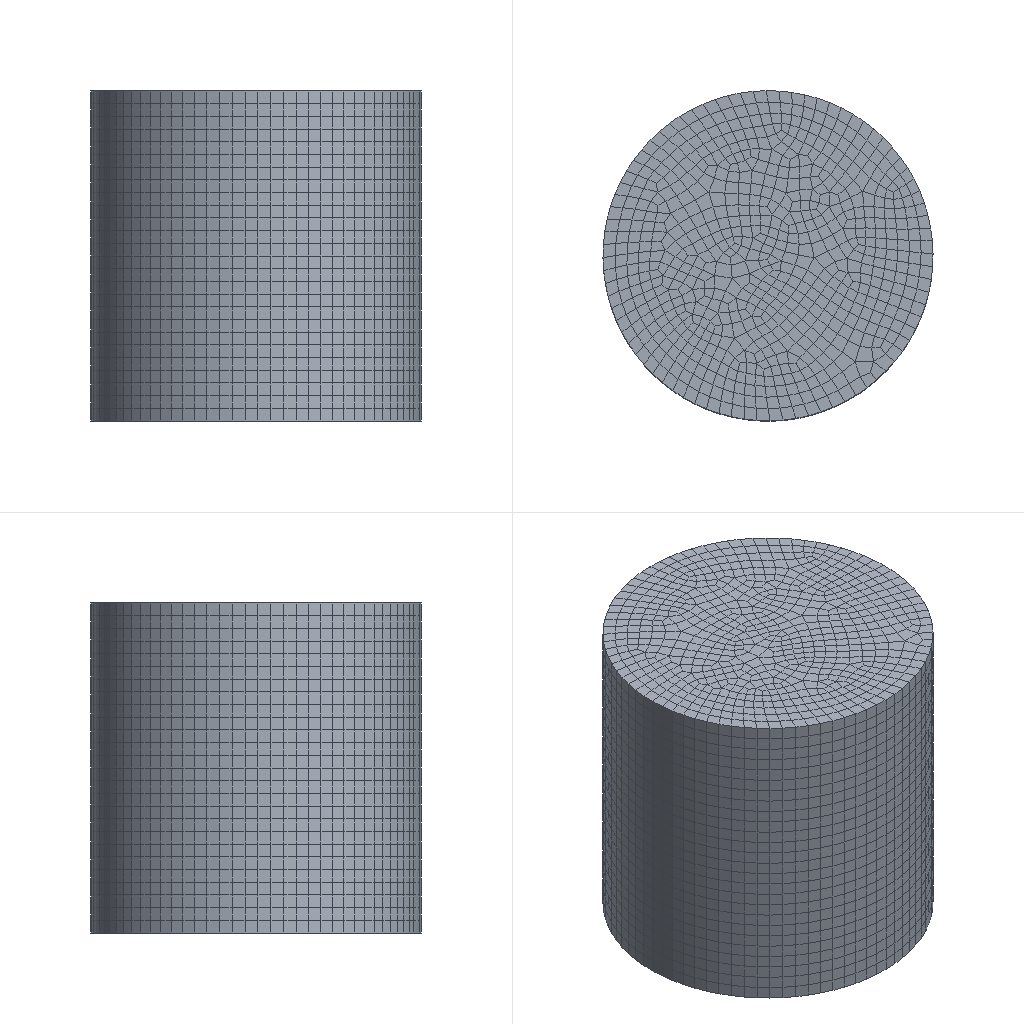Simulation study | abaqus
Set-up summary:
category,name,step,type,value,unit,region
solver,abaqus
solver,version,,,Abaqus/Standard 2020
units,not stated in the deck,,not stated
analysis,deck,,static,static
load_step,Step-1,Step-1,static
load_step,requested,,,1
mesh,nodes,,,20804
mesh,elements,,,18954
element_type,C3D8R,,solid,18252
element_type,COH3D8,,cohesive,702
load,load commands in deck,,count,1
bc,support commands in deck,,count,12
material,COH,,in results
material,MATERIAL-1,,in results
check,setup vs results,,match,"per instance, exact: element labels, types and connectivity; labels of the nodes the elements use; coordinates of those nodes at SINGLE_PRECISION in 1 of 1 instance(s)"
Abaqus input file, long lists of numbers shortened:
*Heading
** Job name: Job-1 Model name: Model-1
** Generated by: Abaqus/CAE 2020
*Preprint, echo=NO, model=NO, history=NO, contact=NO
**
** PARTS
**
*Part, name=Part-1
*Node
      1,   19.206,  -16.005,          25.
      2,   19.206,  -16.005,          50.
** (20802 more lines like these left out)
*Element, type=C3D8R
   1,  1575,  4160,  4244,  1574, 20062, 20063, 20064, 20065
   2,  4161,  1577,  1578,  4162, 20066, 20067, 20068, 20069
** (18250 more lines like these left out)
*Element, type=COH3D8
18253,    10,   335,   251,    11, 20065, 20064, 20063, 20062
18254,   253,    14,    13,   252, 20069, 20068, 20067, 20066
** (700 more lines like these left out)
*Nset, nset=Set-1, generate
     1,  20804,      1
*Elset, elset=Set-1, generate
     1,  18252,      1
*Elset, elset=CohesiveSeam-1-Elements, generate
 18253,  18954,      1
*Nset, nset=CohesiveSeam-1-TopNodes, generate
 20062,  20804,      1
*Nset, nset=CohesiveSeam-1-BottomNodes
   1,   4,   5,   6,   7,   8,   9,  10,  11,  12,  13,  14,  15,  16,  17,  18
  19,  20,  21,  22,  23,  24,  25,  26,  27,  28,  29,  30,  31,  32,  33,  34
** (45 more lines like these left out)
*Elset, elset=__PickedSurf8_S1, internal, generate
 18253,  18954,      1
*Surface, type=ELEMENT, name=_PickedSurf8, internal
__PickedSurf8_S1, S1
*Elset, elset=_CohesiveSeam-1-TopSurf_S2, internal, generate
 18253,  18954,      1
*Surface, type=ELEMENT, name=CohesiveSeam-1-TopSurf
_CohesiveSeam-1-TopSurf_S2, S2
*Elset, elset=_CohesiveSeam-1-BottomSurf_S1, internal, generate
 18253,  18954,      1
*Surface, type=ELEMENT, name=CohesiveSeam-1-BottomSurf
_CohesiveSeam-1-BottomSurf_S1, S1
** Section: Section-1
*Solid Section, elset=Set-1, material=Material-1
,
** Section: coh
*Cohesive Section, elset=CohesiveSeam-1-Elements, controls=EC-1, material=coh, response=TRACTION SEPARATION
,
*End Part
**
**
** ASSEMBLY
**
*Assembly, name=Assembly
**
*Instance, name=Part-1-1, part=Part-1
*End Instance
**
*Node
      1,           0., 1.53080845e-15,           0.
*Nset, nset=Set-1, instance=Part-1-1
    1,    3,    4,    5,    6,    7,    8,    9,   10,   11,   12,   13,   14,   15,   16,   17
   18,   19,   20,   21,   22,   23,   24,   25,   26,   27,   28,   29,   30,   31,   32,   33
** (68 more lines like these left out)
*Elset, elset=Set-1, instance=Part-1-1
  9127,  9128,  9129,  9130,  9131,  9132,  9133,  9134,  9136,  9137,  9138,  9140,  9141,  9143,  9144,  9145
  9147,  9148,  9150,  9151,  9152,  9153,  9154,  9155,  9156,  9159,  9160,  9162,  9163,  9164,  9166,  9167
** (63 more lines like these left out)
*Nset, nset=Set-2, instance=Part-1-1
     2,    83,    84,    85,    86,    87,    88,    89,    90,    91,    92,    93,    94,    95,    96,    97
    98,    99,   100,   101,   102,   103,   104,   105,   106,   107,   108,   109,   110,   111,   112,   113
** (68 more lines like these left out)
*Elset, elset=Set-2, instance=Part-1-1
    1,    2,    3,    4,    5,    6,    7,    8,   10,   11,   12,   14,   15,   17,   18,   19
   21,   22,   24,   25,   26,   27,   28,   29,   30,   33,   34,   36,   37,   38,   40,   41
** (63 more lines like these left out)
*Nset, nset=Set-3, instance=Part-1-1
    3,  162,  163,  164,  165,  166,  167,  168,  169,  170,  171,  172,  173,  174,  175,  176
  177,  178,  179,  180,  181,  182,  183,  184,  185,  186,  187,  188,  189,  190,  191,  192
** (45 more lines like these left out)
*Elset, elset=Set-3, instance=Part-1-1, generate
 17551,  18252,      1
*Nset, nset=Set-5
 1,
*Nset, nset=Set-6, instance=Part-1-1, generate
     1,  20804,      1
*Nset, nset=Set-6
 1,
*Elset, elset=Set-6, instance=Part-1-1, generate
     1,  18954,      1
*Nset, nset=m_Set-4
 1,
*Elset, elset=_s_Surf-1_S2, internal, instance=Part-1-1, generate
 17551,  18252,      1
*Surface, type=ELEMENT, name=s_Surf-1
_s_Surf-1_S2, S2
** Constraint: Constraint-1
*Coupling, constraint name=Constraint-1, ref node=m_Set-4, surface=s_Surf-1
*Kinematic
*Elset, elset=__Int-2_gcs0_2_S6, internal, instance=Part-1-1
    1,    4,   10,   11,   14,   18,   19,   22,   26,   33,   34,   40,   41,   44,   47,   48
   50,   51,   56,   57,   61,   63,   65,   83,  168,  703,  706,  712,  713,  716,  720,  721
** (19 more lines like these left out)
*Elset, elset=__Int-2_gcs0_2_S4, internal, instance=Part-1-1
    2,    3,    5,    6,    7,    8,   12,   15,   17,   21,   24,   25,   27,   28,   29,   30
   36,   37,   38,   42,   45,   46,   52,   53,   58,   60,   62,   64,   69,   70,   71,   72
** (43 more lines like these left out)
*Surface, type=ELEMENT, name=_Int-2_gcs0_2, internal
__Int-2_gcs0_2_S6, S6
__Int-2_gcs0_2_S4, S4
*Elset, elset=__Int-2_gcs0_3_S6, internal, instance=Part-1-1
  9127,  9130,  9136,  9137,  9140,  9144,  9145,  9148,  9152,  9159,  9160,  9166,  9167,  9170,  9173,  9174
  9176,  9177,  9182,  9183,  9187,  9189,  9191,  9209,  9294,  9829,  9832,  9838,  9839,  9842,  9846,  9847
** (19 more lines like these left out)
*Elset, elset=__Int-2_gcs0_3_S4, internal, instance=Part-1-1
  9128,  9129,  9131,  9132,  9133,  9134,  9138,  9141,  9143,  9147,  9150,  9151,  9153,  9154,  9155,  9156
  9162,  9163,  9164,  9168,  9171,  9172,  9178,  9179,  9184,  9186,  9188,  9190,  9195,  9196,  9197,  9198
** (43 more lines like these left out)
*Surface, type=ELEMENT, name=_Int-2_gcs0_3, internal
__Int-2_gcs0_3_S6, S6
__Int-2_gcs0_3_S4, S4
*End Assembly
**
** ELEMENT CONTROLS
**
*Section Controls, name=EC-1, ELEMENT DELETION=YES, VISCOSITY=0.01
1., 1., 1.
*Amplitude, name=Amp-1
             0.,              0.,              1.,              1.
**
** MATERIALS
**
*Material, name=Material-1
*Conductivity
5.,
*Density
 2.7e-09,
*Elastic
32500., 0.2
*Expansion
 1e-06,
*Gap Flow
 0.001,
*Permeability, specific=10.
 0.004, 0.2
*Specific Heat
 9.7e+08,
*Concrete Damaged Plasticity
30.,   0.1,  1.16, 0.667,  0.01
*Concrete Compression Hardening
 31.839,          0.
  35.238, 0.0001688
  37.656, 0.0002734
 39.058, 0.0004092
    39.5, 0.0005746
 38.815, 0.0007747
 37.101,  0.001006
  34.823,  0.001256
 32.332,  0.001511
 29.849,  0.001767
 27.497,  0.002018
 25.334,   0.002263
 23.376,  0.002503
 21.619,  0.002736
 20.051,  0.002963
 18.651,  0.003185
 17.402,  0.003403
 16.285,  0.003616
 15.284,  0.003826
 14.385,   0.004032
 13.573,  0.004236
 12.839,  0.004438
 12.173,  0.004637
 11.567,   0.004835
  11.013,  0.005031
*Concrete Tension Stiffening
  2.09,       0.
   2.4, 8.74e-06
  2.67, 1.23e-05
  2.86, 1.81e-05
  2.94, 2.75e-05
   2.8, 4.37e-05
  2.55, 6.31e-05
   2.3, 8.27e-05
  2.07, 0.000102
  1.86,  0.00012
  1.69, 0.000137
  1.55, 0.000153
  1.42, 0.000169
  1.31, 0.000184
  1.22, 0.000198
  1.14, 0.000213
  1.07, 0.000227
  1.01,  0.00024
 0.956, 0.000254
 0.908, 0.000267
 0.864,  0.00028
 0.825, 0.000293
 0.789, 0.000306
 0.757, 0.000319
 0.727, 0.000332
*Concrete Compression Damage
        0.,          0.
 0.06977, 0.0001688
  0.1005, 0.0002734
  0.1363, 0.0004092
  0.176, 0.0005746
  0.2212, 0.0007747
  0.271,  0.001006
  0.3214,  0.001256
  0.3699,  0.001511
  0.4151,  0.001767
  0.4565,  0.002018
  0.4939,   0.002263
  0.5275,  0.002503
   0.5577,  0.002736
  0.5849,  0.002963
   0.6093,  0.003185
  0.6313,  0.003403
  0.6511,  0.003616
  0.6691,  0.003826
  0.6855,   0.004032
  0.7004,  0.004236
  0.7141,  0.004438
  0.7266,  0.004637
  0.7382,   0.004835
  0.7488,  0.005031
  0.7586,  0.005226
  0.7678,  0.005419
  0.7763,  0.005611
  0.7842,  0.005802
  0.7915,  0.005993
  0.7984,  0.006182
  0.8049,  0.006371
  0.811,  0.006559
  0.8167,  0.006747
  0.8221,  0.006933
  0.8627,  0.008781
  0.8884,   0.01061
  0.906,   0.01242
  0.9188,   0.01423
  0.9286,   0.01603
** (21 more lines like these left out)
*Concrete Tension Damage, compression recovery=0.45
     0.,       0.
 0.0544, 8.74e-06
 0.0674, 1.23e-05
 0.0893, 1.81e-05
  0.124, 2.75e-05
  0.186, 4.37e-05
  0.255, 6.31e-05
  0.321, 8.27e-05
   0.38, 0.000102
  0.431,  0.00012
  0.475, 0.000137
  0.513, 0.000153
  0.546, 0.000169
  0.575, 0.000184
  0.601, 0.000198
  0.623, 0.000213
  0.643, 0.000227
  0.661,  0.00024
  0.678, 0.000254
  0.692, 0.000267
  0.706,  0.00028
  0.718, 0.000293
  0.729, 0.000306
  0.739, 0.000319
  0.749, 0.000332
  0.757, 0.000344
  0.765, 0.000357
  0.773, 0.000369
   0.78, 0.000382
  0.787, 0.000394
  0.793, 0.000407
  0.799, 0.000419
  0.804, 0.000431
  0.809, 0.000443
  0.814, 0.000456
  0.851, 0.000577
  0.875, 0.000697
  0.892, 0.000816
  0.905, 0.000935
  0.915,  0.00105
** (31 more lines like these left out)
*Material, name=coh
*Damage Initiation, criterion=MAXS
15.,15.,15.
*Damage Evolution, type=DISPLACEMENT
 1e-11,
*Damage Stabilization
0.01
*Density
 2.7e-09,
*Elastic, type=TRACTION
20000.,20000.,20000.
**
** INTERACTION PROPERTIES
**
*Surface Interaction, name=IntProp-1
1.,
*Friction, slip tolerance=0.005
 0.1,
*Surface Behavior, pressure-overclosure=HARD
**
** PREDEFINED FIELDS
**
** Name: Predefined Field-1   Type: Void ratio
*Initial Conditions, TYPE=RATIO
Set-6, 0.1
**
** INTERACTIONS
**
** Interaction: Int-2
*Contact
*Contact Inclusions, ALL EXTERIOR
*Contact Property Assignment
 ,  , IntProp-1
*Surface Property Assignment, property=GEOMETRIC CORRECTION
_Int-2_gcs0_2, Circumferential, 0., 0., 0.,  0., 0., 1.
_Int-2_gcs0_3, Circumferential, 0., 0., 0.,  0., 0., 1.
** ----------------------------------------------------------------
**
** STEP: Step-1
**
*Step, name=Step-1, nlgeom=YES, inc=1000
*Static, stabilize=0.0002, allsdtol=0.05, continue=NO
0.01, 1., 1e-09, 1.
**
** BOUNDARY CONDITIONS
**
** Name: BC-1 Type: 位移/转角
*Boundary
Set-5, 1, 1
Set-5, 2, 2
Set-5, 3, 3
Set-5, 4, 4
Set-5, 5, 5
Set-5, 6, 6
** Name: BC-2 Type: 位移/转角
*Boundary, amplitude=Amp-1
Set-2, 1, 1, 2.
Set-2, 2, 2
Set-2, 3, 3
Set-2, 4, 4
Set-2, 5, 5
Set-2, 6, 6
**
** CONTROLS
**
*Controls, reset
*Controls, parameters=time incrementation
, , , , , , , 15, , ,
**
** OUTPUT REQUESTS
**
*Restart, write, number interval=1, time marks=NO
**
** FIELD OUTPUT: F-Output-1
**
*Output, field
*Node Output
RF, RM, RT, U, V
*Element Output, directions=YES
DAMAGEC, DAMAGET, E, LE, MISES, MISESMAX, PE, PEEQ, S, SDEG, STATUS
*Contact Output
CDISP, CSTRESS
**
** HISTORY OUTPUT: H-Output-1
**
*Output, history
*Node Output, nset=Set-5
RF1, RF2, U1, U2
*End Step
Results summary:
result,step,,partial,increments=123 time=0.005496/1.0
result,analysis,,,static
result,last_loadstep,,,1
result,primary field,,,U
result,reaction total,,FX,42.003,model units
result,reaction total,,FY,-0.4249,model units
result,reaction total,,FZ,-4.179,model units